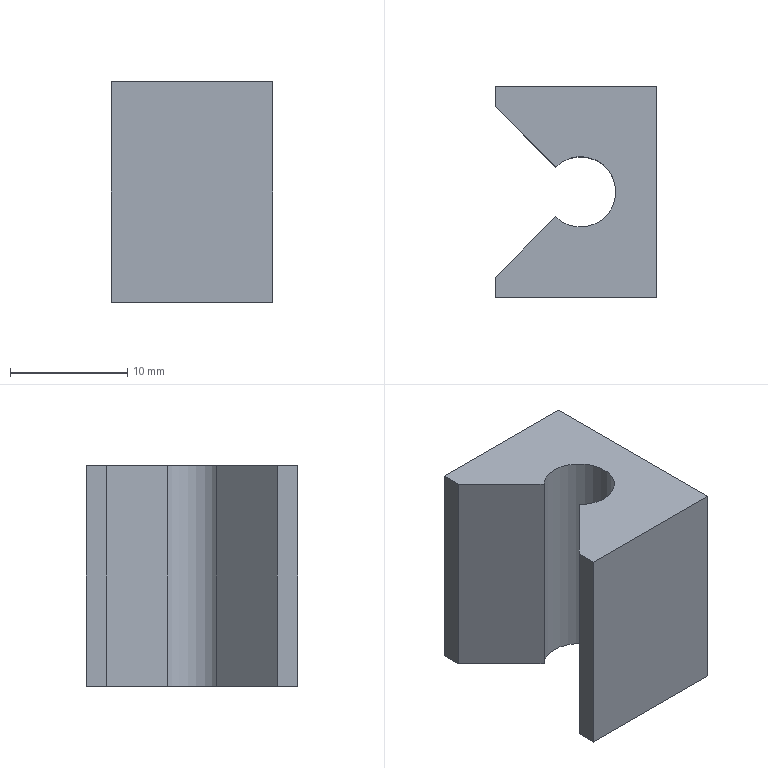Part | NX | features solid 2 | 1 solid | 10 faces | box 13.775 x 18 x 18.75 mm | volume 3258 mm3 | plane 9 | cylinder 1 | commonest cylinder face diameters 6 x1
STEP:
#1=CARTESIAN_POINT('',(125.298,-51.7,-47.));
#2=VERTEX_POINT('',#1);
#3=CARTESIAN_POINT('',(111.523,-51.7,-47.));
#4=VERTEX_POINT('',#3);
#5=CARTESIAN_POINT('',(103.023,-51.7,-47.));
#6=DIRECTION('',(-1.,0.,0.));
#7=VECTOR('',#6,1000.);
#8=LINE('',#5,#7);
#9=EDGE_CURVE('',#2,#4,#8,.T.);
#10=ORIENTED_EDGE('',*,*,#9,.T.);
#11=CARTESIAN_POINT('',(111.523,-51.7,-65.75));
#12=VERTEX_POINT('',#11);
#13=CARTESIAN_POINT('',(111.523,-51.7,-103.25));
#14=DIRECTION('',(0.,0.,-1.));
#15=VECTOR('',#14,1000.);
#16=LINE('',#13,#15);
#17=EDGE_CURVE('',#4,#12,#16,.T.);
#18=ORIENTED_EDGE('',*,*,#17,.T.);
#19=CARTESIAN_POINT('',(125.298,-51.7,-65.75));
#20=VERTEX_POINT('',#19);
#21=CARTESIAN_POINT('',(103.023,-51.7,-65.75));
#22=DIRECTION('',(1.,0.,0.));
#23=VECTOR('',#22,1000.);
#24=LINE('',#21,#23);
#25=EDGE_CURVE('',#12,#20,#24,.T.);
#26=ORIENTED_EDGE('',*,*,#25,.T.);
#27=CARTESIAN_POINT('',(125.298,-51.7,-47.));
#28=DIRECTION('',(0.,0.,-1.));
#29=VECTOR('',#28,1000.);
#30=LINE('',#27,#29);
#31=EDGE_CURVE('',#2,#20,#30,.T.);
#32=ORIENTED_EDGE('',*,*,#31,.F.);
#33=EDGE_LOOP('',(#10,#18,#26,#32));
#34=FACE_BOUND('',#33,.T.);
#35=CARTESIAN_POINT('',(103.023,-51.7,-47.));
#36=DIRECTION('',(0.,-1.,0.));
#37=DIRECTION('',(0.,0.,1.));
#38=AXIS2_PLACEMENT_3D('',#35,#36,#37);
#39=PLANE('',#38);
#40=ADVANCED_FACE('',(#34),#39,.T.);
#41=CARTESIAN_POINT('',(125.298,-33.7,-65.75));
#42=VERTEX_POINT('',#41);
#43=CARTESIAN_POINT('',(111.523,-33.7,-65.75));
#44=VERTEX_POINT('',#43);
#45=CARTESIAN_POINT('',(103.023,-33.7,-65.75));
#46=DIRECTION('',(-1.,0.,0.));
#47=VECTOR('',#46,1000.);
#48=LINE('',#45,#47);
#49=EDGE_CURVE('',#42,#44,#48,.T.);
#50=ORIENTED_EDGE('',*,*,#49,.T.);
#51=CARTESIAN_POINT('',(111.523,-33.7,-47.));
#52=VERTEX_POINT('',#51);
#53=CARTESIAN_POINT('',(111.523,-33.7,-103.25));
#54=DIRECTION('',(0.,0.,1.));
#55=VECTOR('',#54,1000.);
#56=LINE('',#53,#55);
#57=EDGE_CURVE('',#44,#52,#56,.T.);
#58=ORIENTED_EDGE('',*,*,#57,.T.);
#59=CARTESIAN_POINT('',(125.298,-33.7,-47.));
#60=VERTEX_POINT('',#59);
#61=CARTESIAN_POINT('',(103.023,-33.7,-47.));
#62=DIRECTION('',(1.,0.,0.));
#63=VECTOR('',#62,1000.);
#64=LINE('',#61,#63);
#65=EDGE_CURVE('',#52,#60,#64,.T.);
#66=ORIENTED_EDGE('',*,*,#65,.T.);
#67=CARTESIAN_POINT('',(125.298,-33.7,-47.));
#68=DIRECTION('',(0.,0.,-1.));
#69=VECTOR('',#68,1000.);
#70=LINE('',#67,#69);
#71=EDGE_CURVE('',#60,#42,#70,.T.);
#72=ORIENTED_EDGE('',*,*,#71,.T.);
#73=EDGE_LOOP('',(#50,#58,#66,#72));
#74=FACE_BOUND('',#73,.T.);
#75=CARTESIAN_POINT('',(103.023,-33.7,-47.));
#76=DIRECTION('',(0.,1.,0.));
#77=DIRECTION('',(0.,0.,-1.));
#78=AXIS2_PLACEMENT_3D('',#75,#76,#77);
#79=PLANE('',#78);
#80=ADVANCED_FACE('',(#74),#79,.T.);
#81=CARTESIAN_POINT('',(111.523,-35.422,-65.75));
#82=VERTEX_POINT('',#81);
#83=CARTESIAN_POINT('',(111.523,-42.7,-65.75));
#84=DIRECTION('',(0.,-1.,0.));
#85=VECTOR('',#84,1000.);
#86=LINE('',#83,#85);
#87=EDGE_CURVE('',#44,#82,#86,.T.);
#88=ORIENTED_EDGE('',*,*,#87,.F.);
#89=ORIENTED_EDGE('',*,*,#49,.F.);
#90=CARTESIAN_POINT('',(125.298,-42.7,-65.75));
#91=DIRECTION('',(0.,1.,0.));
#92=VECTOR('',#91,1000.);
#93=LINE('',#90,#92);
#94=EDGE_CURVE('',#20,#42,#93,.T.);
#95=ORIENTED_EDGE('',*,*,#94,.F.);
#96=ORIENTED_EDGE('',*,*,#25,.F.);
#97=CARTESIAN_POINT('',(111.523,-49.978,-65.75));
#98=VERTEX_POINT('',#97);
#99=CARTESIAN_POINT('',(111.523,-42.7,-65.75));
#100=DIRECTION('',(0.,-1.,0.));
#101=VECTOR('',#100,1000.);
#102=LINE('',#99,#101);
#103=EDGE_CURVE('',#98,#12,#102,.T.);
#104=ORIENTED_EDGE('',*,*,#103,.F.);
#105=CARTESIAN_POINT('',(116.68,-44.821,-65.75));
#106=VERTEX_POINT('',#105);
#107=CARTESIAN_POINT('',(114.913,-46.589,-65.75));
#108=DIRECTION('',(-0.7071,-0.7071,0.));
#109=VECTOR('',#108,1000.);
#110=LINE('',#107,#109);
#111=EDGE_CURVE('',#106,#98,#110,.T.);
#112=ORIENTED_EDGE('',*,*,#111,.F.);
#113=CARTESIAN_POINT('',(116.68,-40.579,-65.75));
#114=VERTEX_POINT('',#113);
#115=CARTESIAN_POINT('',(118.802,-42.7,-65.75));
#116=DIRECTION('',(0.,0.,-1.));
#117=DIRECTION('',(-1.,0.,0.));
#118=AXIS2_PLACEMENT_3D('',#115,#116,#117);
#119=CIRCLE('',#118,3.);
#120=EDGE_CURVE('',#114,#106,#119,.T.);
#121=ORIENTED_EDGE('',*,*,#120,.F.);
#122=CARTESIAN_POINT('',(114.913,-38.811,-65.75));
#123=DIRECTION('',(0.7071,-0.7071,0.));
#124=VECTOR('',#123,1000.);
#125=LINE('',#122,#124);
#126=EDGE_CURVE('',#82,#114,#125,.T.);
#127=ORIENTED_EDGE('',*,*,#126,.F.);
#128=EDGE_LOOP('',(#88,#89,#95,#96,#104,#112,#121,#127));
#129=FACE_BOUND('',#128,.T.);
#130=CARTESIAN_POINT('',(103.023,-42.7,-65.75));
#131=DIRECTION('',(0.,0.,-1.));
#132=DIRECTION('',(-1.,0.,0.));
#133=AXIS2_PLACEMENT_3D('',#130,#131,#132);
#134=PLANE('',#133);
#135=ADVANCED_FACE('',(#129),#134,.T.);
#136=ORIENTED_EDGE('',*,*,#31,.T.);
#137=ORIENTED_EDGE('',*,*,#94,.T.);
#138=ORIENTED_EDGE('',*,*,#71,.F.);
#139=CARTESIAN_POINT('',(125.298,-42.7,-47.));
#140=DIRECTION('',(0.,-1.,0.));
#141=VECTOR('',#140,1000.);
#142=LINE('',#139,#141);
#143=EDGE_CURVE('',#60,#2,#142,.T.);
#144=ORIENTED_EDGE('',*,*,#143,.T.);
#145=EDGE_LOOP('',(#136,#137,#138,#144));
#146=FACE_BOUND('',#145,.T.);
#147=CARTESIAN_POINT('',(125.298,-42.7,-47.));
#148=DIRECTION('',(1.,0.,0.));
#149=DIRECTION('',(0.,0.,-1.));
#150=AXIS2_PLACEMENT_3D('',#147,#148,#149);
#151=PLANE('',#150);
#152=ADVANCED_FACE('',(#146),#151,.T.);
#153=CARTESIAN_POINT('',(111.523,-49.978,-47.));
#154=VERTEX_POINT('',#153);
#155=CARTESIAN_POINT('',(111.523,-42.7,-47.));
#156=DIRECTION('',(0.,1.,0.));
#157=VECTOR('',#156,1000.);
#158=LINE('',#155,#157);
#159=EDGE_CURVE('',#4,#154,#158,.T.);
#160=ORIENTED_EDGE('',*,*,#159,.F.);
#161=ORIENTED_EDGE('',*,*,#9,.F.);
#162=ORIENTED_EDGE('',*,*,#143,.F.);
#163=ORIENTED_EDGE('',*,*,#65,.F.);
#164=CARTESIAN_POINT('',(111.523,-35.422,-47.));
#165=VERTEX_POINT('',#164);
#166=CARTESIAN_POINT('',(111.523,-42.7,-47.));
#167=DIRECTION('',(0.,1.,0.));
#168=VECTOR('',#167,1000.);
#169=LINE('',#166,#168);
#170=EDGE_CURVE('',#165,#52,#169,.T.);
#171=ORIENTED_EDGE('',*,*,#170,.F.);
#172=CARTESIAN_POINT('',(116.68,-40.579,-47.));
#173=VERTEX_POINT('',#172);
#174=CARTESIAN_POINT('',(114.913,-38.811,-47.));
#175=DIRECTION('',(-0.7071,0.7071,0.));
#176=VECTOR('',#175,1000.);
#177=LINE('',#174,#176);
#178=EDGE_CURVE('',#173,#165,#177,.T.);
#179=ORIENTED_EDGE('',*,*,#178,.F.);
#180=CARTESIAN_POINT('',(116.68,-44.821,-47.));
#181=VERTEX_POINT('',#180);
#182=CARTESIAN_POINT('',(118.802,-42.7,-47.));
#183=DIRECTION('',(0.,0.,1.));
#184=DIRECTION('',(1.,0.,0.));
#185=AXIS2_PLACEMENT_3D('',#182,#183,#184);
#186=CIRCLE('',#185,3.);
#187=EDGE_CURVE('',#181,#173,#186,.T.);
#188=ORIENTED_EDGE('',*,*,#187,.F.);
#189=CARTESIAN_POINT('',(114.913,-46.589,-47.));
#190=DIRECTION('',(0.7071,0.7071,0.));
#191=VECTOR('',#190,1000.);
#192=LINE('',#189,#191);
#193=EDGE_CURVE('',#154,#181,#192,.T.);
#194=ORIENTED_EDGE('',*,*,#193,.F.);
#195=EDGE_LOOP('',(#160,#161,#162,#163,#171,#179,#188,#194));
#196=FACE_BOUND('',#195,.T.);
#197=CARTESIAN_POINT('',(103.023,-42.7,-47.));
#198=DIRECTION('',(0.,0.,1.));
#199=DIRECTION('',(1.,0.,0.));
#200=AXIS2_PLACEMENT_3D('',#197,#198,#199);
#201=PLANE('',#200);
#202=ADVANCED_FACE('',(#196),#201,.T.);
#203=ORIENTED_EDGE('',*,*,#111,.T.);
#204=CARTESIAN_POINT('',(111.523,-49.978,-35.75));
#205=DIRECTION('',(0.,0.,1.));
#206=VECTOR('',#205,1000.);
#207=LINE('',#204,#206);
#208=EDGE_CURVE('',#98,#154,#207,.T.);
#209=ORIENTED_EDGE('',*,*,#208,.T.);
#210=ORIENTED_EDGE('',*,*,#193,.T.);
#211=CARTESIAN_POINT('',(116.68,-44.821,-32.75));
#212=DIRECTION('',(0.,0.,-1.));
#213=VECTOR('',#212,1000.);
#214=LINE('',#211,#213);
#215=EDGE_CURVE('',#181,#106,#214,.T.);
#216=ORIENTED_EDGE('',*,*,#215,.T.);
#217=EDGE_LOOP('',(#203,#209,#210,#216));
#218=FACE_BOUND('',#217,.T.);
#219=CARTESIAN_POINT('',(114.913,-46.589,-35.75));
#220=DIRECTION('',(0.7071,-0.7071,0.));
#221=DIRECTION('',(-0.7071,-0.7071,0.));
#222=AXIS2_PLACEMENT_3D('',#219,#220,#221);
#223=PLANE('',#222);
#224=ADVANCED_FACE('',(#218),#223,.F.);
#225=ORIENTED_EDGE('',*,*,#126,.T.);
#226=CARTESIAN_POINT('',(116.68,-40.579,-32.75));
#227=DIRECTION('',(0.,0.,-1.));
#228=VECTOR('',#227,1000.);
#229=LINE('',#226,#228);
#230=EDGE_CURVE('',#114,#173,#229,.F.);
#231=ORIENTED_EDGE('',*,*,#230,.T.);
#232=ORIENTED_EDGE('',*,*,#178,.T.);
#233=CARTESIAN_POINT('',(111.523,-35.422,-103.25));
#234=DIRECTION('',(0.,0.,1.));
#235=VECTOR('',#234,1000.);
#236=LINE('',#233,#235);
#237=EDGE_CURVE('',#82,#165,#236,.T.);
#238=ORIENTED_EDGE('',*,*,#237,.F.);
#239=EDGE_LOOP('',(#225,#231,#232,#238));
#240=FACE_BOUND('',#239,.T.);
#241=CARTESIAN_POINT('',(114.913,-38.811,-35.75));
#242=DIRECTION('',(0.7071,0.7071,0.));
#243=DIRECTION('',(0.7071,-0.7071,0.));
#244=AXIS2_PLACEMENT_3D('',#241,#242,#243);
#245=PLANE('',#244);
#246=ADVANCED_FACE('',(#240),#245,.F.);
#247=ORIENTED_EDGE('',*,*,#120,.T.);
#248=ORIENTED_EDGE('',*,*,#215,.F.);
#249=ORIENTED_EDGE('',*,*,#187,.T.);
#250=ORIENTED_EDGE('',*,*,#230,.F.);
#251=EDGE_LOOP('',(#247,#248,#249,#250));
#252=FACE_BOUND('',#251,.T.);
#253=CARTESIAN_POINT('',(118.802,-42.7,-32.75));
#254=DIRECTION('',(0.,0.,-1.));
#255=DIRECTION('',(-1.,0.,0.));
#256=AXIS2_PLACEMENT_3D('',#253,#254,#255);
#257=CYLINDRICAL_SURFACE('',#256,3.);
#258=ADVANCED_FACE('',(#252),#257,.F.);
#259=ORIENTED_EDGE('',*,*,#87,.T.);
#260=ORIENTED_EDGE('',*,*,#237,.T.);
#261=ORIENTED_EDGE('',*,*,#170,.T.);
#262=ORIENTED_EDGE('',*,*,#57,.F.);
#263=EDGE_LOOP('',(#259,#260,#261,#262));
#264=FACE_BOUND('',#263,.T.);
#265=CARTESIAN_POINT('',(111.523,-51.7,-103.25));
#266=DIRECTION('',(1.,0.,0.));
#267=DIRECTION('',(0.,0.,-1.));
#268=AXIS2_PLACEMENT_3D('',#265,#266,#267);
#269=PLANE('',#268);
#270=ADVANCED_FACE('',(#264),#269,.F.);
#271=ORIENTED_EDGE('',*,*,#103,.T.);
#272=ORIENTED_EDGE('',*,*,#17,.F.);
#273=ORIENTED_EDGE('',*,*,#159,.T.);
#274=ORIENTED_EDGE('',*,*,#208,.F.);
#275=EDGE_LOOP('',(#271,#272,#273,#274));
#276=FACE_BOUND('',#275,.T.);
#277=CARTESIAN_POINT('',(111.523,-51.7,-103.25));
#278=DIRECTION('',(1.,0.,0.));
#279=DIRECTION('',(0.,0.,-1.));
#280=AXIS2_PLACEMENT_3D('',#277,#278,#279);
#281=PLANE('',#280);
#282=ADVANCED_FACE('',(#276),#281,.F.);
#283=CLOSED_SHELL('',(#40,#80,#135,#152,#202,#224,#246,#258,#270,#282));
#284=MANIFOLD_SOLID_BREP('',#283);
#285=(LENGTH_UNIT()NAMED_UNIT(*)SI_UNIT(.MILLI.,.METRE.));
#286=UNCERTAINTY_MEASURE_WITH_UNIT(LENGTH_MEASURE(0.00001),#285,'','');
#287=(NAMED_UNIT(*)PLANE_ANGLE_UNIT()SI_UNIT($,.RADIAN.));
#288=(NAMED_UNIT(*)SI_UNIT($,.STERADIAN.)SOLID_ANGLE_UNIT());
#289=(GEOMETRIC_REPRESENTATION_CONTEXT(3)GLOBAL_UNCERTAINTY_ASSIGNED_CONTEXT((#286))GLOBAL_UNIT_ASSIGNED_CONTEXT((#285,#287,#288))REPRESENTATION_CONTEXT('',''));
#290=ADVANCED_BREP_SHAPE_REPRESENTATION('',(#284),#289);